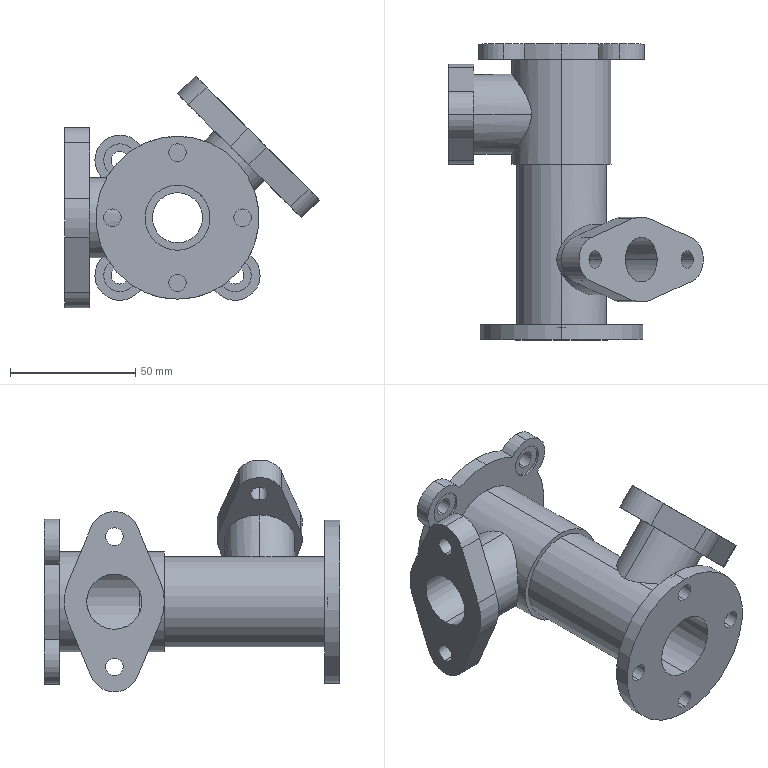Part | SolidWorks | features ICE 20, Extrusion 1 | 1 solid | 114 faces | box 101.569 x 118 x 92.569 mm | volume 130273 mm3 | cylinder 85 | plane 29 | commonest cylinder face diameters 7 x24 20 x11 12.5 x8 13 x8 65 x7 18 x5